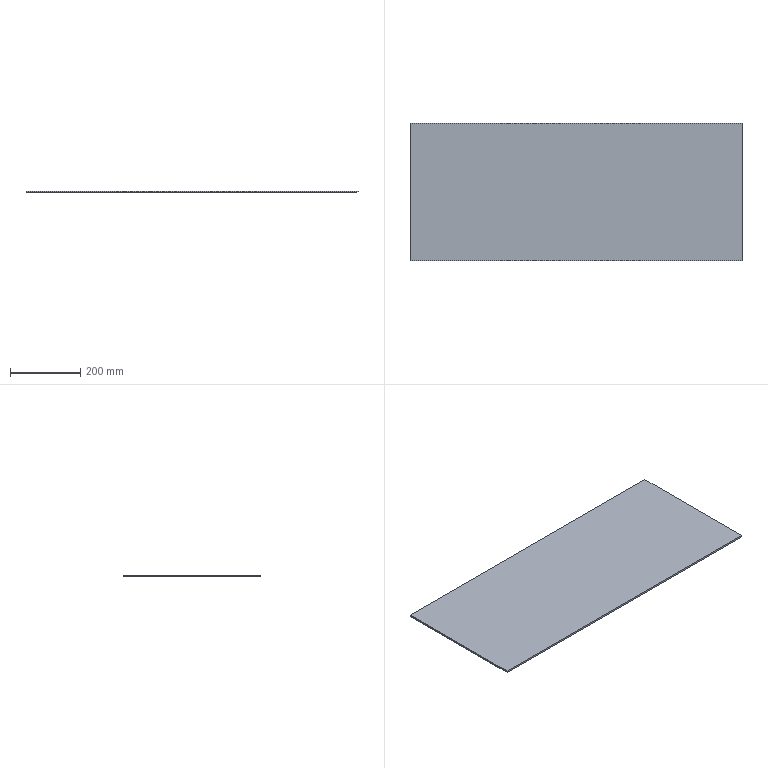Part | SolidWorks | features BaseBody 1 | 1 solid | 6 faces | box 945 x 390 x 5 mm | volume 1837875 mm3 | plane 6
STEP:
#1=CARTESIAN_POINT('',(-472.5,195.,0.));
#2=VERTEX_POINT('',#1);
#3=CARTESIAN_POINT('',(-472.5,-195.,0.));
#4=VERTEX_POINT('',#3);
#5=CARTESIAN_POINT('',(-472.5,-195.,0.));
#6=DIRECTION('',(0.,-1.,0.));
#7=VECTOR('',#6,1000.);
#8=LINE('',#5,#7);
#9=EDGE_CURVE('',#2,#4,#8,.T.);
#10=ORIENTED_EDGE('',*,*,#9,.T.);
#11=CARTESIAN_POINT('',(-472.5,-195.,5.));
#12=VERTEX_POINT('',#11);
#13=CARTESIAN_POINT('',(-472.5,-195.,5.));
#14=DIRECTION('',(0.,0.,-1.));
#15=VECTOR('',#14,1000.);
#16=LINE('',#13,#15);
#17=EDGE_CURVE('',#12,#4,#16,.T.);
#18=ORIENTED_EDGE('',*,*,#17,.F.);
#19=CARTESIAN_POINT('',(-472.5,195.,5.));
#20=VERTEX_POINT('',#19);
#21=CARTESIAN_POINT('',(-472.5,-195.,5.));
#22=DIRECTION('',(0.,-1.,0.));
#23=VECTOR('',#22,1000.);
#24=LINE('',#21,#23);
#25=EDGE_CURVE('',#20,#12,#24,.T.);
#26=ORIENTED_EDGE('',*,*,#25,.F.);
#27=CARTESIAN_POINT('',(-472.5,195.,5.));
#28=DIRECTION('',(0.,0.,-1.));
#29=VECTOR('',#28,1000.);
#30=LINE('',#27,#29);
#31=EDGE_CURVE('',#20,#2,#30,.T.);
#32=ORIENTED_EDGE('',*,*,#31,.T.);
#33=EDGE_LOOP('',(#10,#18,#26,#32));
#34=FACE_OUTER_BOUND('',#33,.T.);
#35=CARTESIAN_POINT('',(-472.5,-195.,5.));
#36=DIRECTION('',(1.,0.,0.));
#37=DIRECTION('',(0.,0.,-1.));
#38=AXIS2_PLACEMENT_3D('',#35,#36,#37);
#39=PLANE('',#38);
#40=ADVANCED_FACE('',(#34),#39,.F.);
#41=CARTESIAN_POINT('',(467.5,-195.,0.));
#42=VERTEX_POINT('',#41);
#43=CARTESIAN_POINT('',(472.5,-195.,0.));
#44=DIRECTION('',(1.,0.,0.));
#45=VECTOR('',#44,1000.);
#46=LINE('',#43,#45);
#47=EDGE_CURVE('',#4,#42,#46,.T.);
#48=ORIENTED_EDGE('',*,*,#47,.T.);
#49=CARTESIAN_POINT('',(472.5,-195.,5.));
#50=VERTEX_POINT('',#49);
#51=CARTESIAN_POINT('',(472.5,-195.,5.));
#52=DIRECTION('',(0.7071,0.,0.7071));
#53=VECTOR('',#52,1000.);
#54=LINE('',#51,#53);
#55=EDGE_CURVE('',#42,#50,#54,.T.);
#56=ORIENTED_EDGE('',*,*,#55,.T.);
#57=CARTESIAN_POINT('',(472.5,-195.,5.));
#58=DIRECTION('',(1.,0.,0.));
#59=VECTOR('',#58,1000.);
#60=LINE('',#57,#59);
#61=EDGE_CURVE('',#12,#50,#60,.T.);
#62=ORIENTED_EDGE('',*,*,#61,.F.);
#63=ORIENTED_EDGE('',*,*,#17,.T.);
#64=EDGE_LOOP('',(#48,#56,#62,#63));
#65=FACE_OUTER_BOUND('',#64,.T.);
#66=CARTESIAN_POINT('',(472.5,-195.,5.));
#67=DIRECTION('',(0.,1.,0.));
#68=DIRECTION('',(-1.,0.,0.));
#69=AXIS2_PLACEMENT_3D('',#66,#67,#68);
#70=PLANE('',#69);
#71=ADVANCED_FACE('',(#65),#70,.F.);
#72=CARTESIAN_POINT('',(472.5,195.,5.));
#73=VERTEX_POINT('',#72);
#74=CARTESIAN_POINT('',(472.5,195.,5.));
#75=DIRECTION('',(-1.,0.,0.));
#76=VECTOR('',#75,1000.);
#77=LINE('',#74,#76);
#78=EDGE_CURVE('',#73,#20,#77,.T.);
#79=ORIENTED_EDGE('',*,*,#78,.F.);
#80=CARTESIAN_POINT('',(467.5,195.,0.));
#81=VERTEX_POINT('',#80);
#82=CARTESIAN_POINT('',(472.5,195.,5.));
#83=DIRECTION('',(-0.7071,0.,-0.7071));
#84=VECTOR('',#83,1000.);
#85=LINE('',#82,#84);
#86=EDGE_CURVE('',#73,#81,#85,.T.);
#87=ORIENTED_EDGE('',*,*,#86,.T.);
#88=CARTESIAN_POINT('',(472.5,195.,0.));
#89=DIRECTION('',(-1.,0.,0.));
#90=VECTOR('',#89,1000.);
#91=LINE('',#88,#90);
#92=EDGE_CURVE('',#81,#2,#91,.T.);
#93=ORIENTED_EDGE('',*,*,#92,.T.);
#94=ORIENTED_EDGE('',*,*,#31,.F.);
#95=EDGE_LOOP('',(#79,#87,#93,#94));
#96=FACE_OUTER_BOUND('',#95,.T.);
#97=CARTESIAN_POINT('',(472.5,195.,5.));
#98=DIRECTION('',(0.,-1.,0.));
#99=DIRECTION('',(1.,0.,0.));
#100=AXIS2_PLACEMENT_3D('',#97,#98,#99);
#101=PLANE('',#100);
#102=ADVANCED_FACE('',(#96),#101,.F.);
#103=ORIENTED_EDGE('',*,*,#25,.T.);
#104=ORIENTED_EDGE('',*,*,#61,.T.);
#105=CARTESIAN_POINT('',(472.5,-195.,5.));
#106=DIRECTION('',(0.,1.,0.));
#107=VECTOR('',#106,1000.);
#108=LINE('',#105,#107);
#109=EDGE_CURVE('',#50,#73,#108,.T.);
#110=ORIENTED_EDGE('',*,*,#109,.T.);
#111=ORIENTED_EDGE('',*,*,#78,.T.);
#112=EDGE_LOOP('',(#103,#104,#110,#111));
#113=FACE_OUTER_BOUND('',#112,.T.);
#114=CARTESIAN_POINT('',(0.,0.,5.));
#115=DIRECTION('',(0.,0.,1.));
#116=DIRECTION('',(1.,0.,0.));
#117=AXIS2_PLACEMENT_3D('',#114,#115,#116);
#118=PLANE('',#117);
#119=ADVANCED_FACE('',(#113),#118,.T.);
#120=ORIENTED_EDGE('',*,*,#92,.F.);
#121=CARTESIAN_POINT('',(467.5,0.,0.));
#122=DIRECTION('',(0.,-1.,0.));
#123=VECTOR('',#122,1000.);
#124=LINE('',#121,#123);
#125=EDGE_CURVE('',#81,#42,#124,.T.);
#126=ORIENTED_EDGE('',*,*,#125,.T.);
#127=ORIENTED_EDGE('',*,*,#47,.F.);
#128=ORIENTED_EDGE('',*,*,#9,.F.);
#129=EDGE_LOOP('',(#120,#126,#127,#128));
#130=FACE_OUTER_BOUND('',#129,.T.);
#131=CARTESIAN_POINT('',(0.,0.,0.));
#132=DIRECTION('',(0.,0.,1.));
#133=DIRECTION('',(1.,0.,0.));
#134=AXIS2_PLACEMENT_3D('',#131,#132,#133);
#135=PLANE('',#134);
#136=ADVANCED_FACE('',(#130),#135,.F.);
#137=ORIENTED_EDGE('',*,*,#55,.F.);
#138=ORIENTED_EDGE('',*,*,#125,.F.);
#139=ORIENTED_EDGE('',*,*,#86,.F.);
#140=ORIENTED_EDGE('',*,*,#109,.F.);
#141=EDGE_LOOP('',(#137,#138,#139,#140));
#142=FACE_OUTER_BOUND('',#141,.T.);
#143=CARTESIAN_POINT('',(472.5,-195.,5.));
#144=DIRECTION('',(-0.7071,0.,0.7071));
#145=DIRECTION('',(0.,1.,0.));
#146=AXIS2_PLACEMENT_3D('',#143,#144,#145);
#147=PLANE('',#146);
#148=ADVANCED_FACE('',(#142),#147,.F.);
#149=CLOSED_SHELL('',(#40,#71,#102,#119,#136,#148));
#150=MANIFOLD_SOLID_BREP('',#149);
#151=CARTESIAN_POINT('',(0.,0.,0.));
#152=DIRECTION('',(0.,0.,1.));
#153=DIRECTION('',(1.,0.,0.));
#154=AXIS2_PLACEMENT_3D('',#151,#152,#153);
#155=(LENGTH_UNIT()NAMED_UNIT(*)SI_UNIT(.MILLI.,.METRE.));
#156=UNCERTAINTY_MEASURE_WITH_UNIT(LENGTH_MEASURE(0.00001),#155,'','');
#157=(NAMED_UNIT(*)PLANE_ANGLE_UNIT()SI_UNIT($,.RADIAN.));
#158=(NAMED_UNIT(*)SI_UNIT($,.STERADIAN.)SOLID_ANGLE_UNIT());
#159=(GEOMETRIC_REPRESENTATION_CONTEXT(3)GLOBAL_UNCERTAINTY_ASSIGNED_CONTEXT((#156))GLOBAL_UNIT_ASSIGNED_CONTEXT((#155,#157,#158))REPRESENTATION_CONTEXT('',''));
#160=ADVANCED_BREP_SHAPE_REPRESENTATION('',(#150,#154),#159);